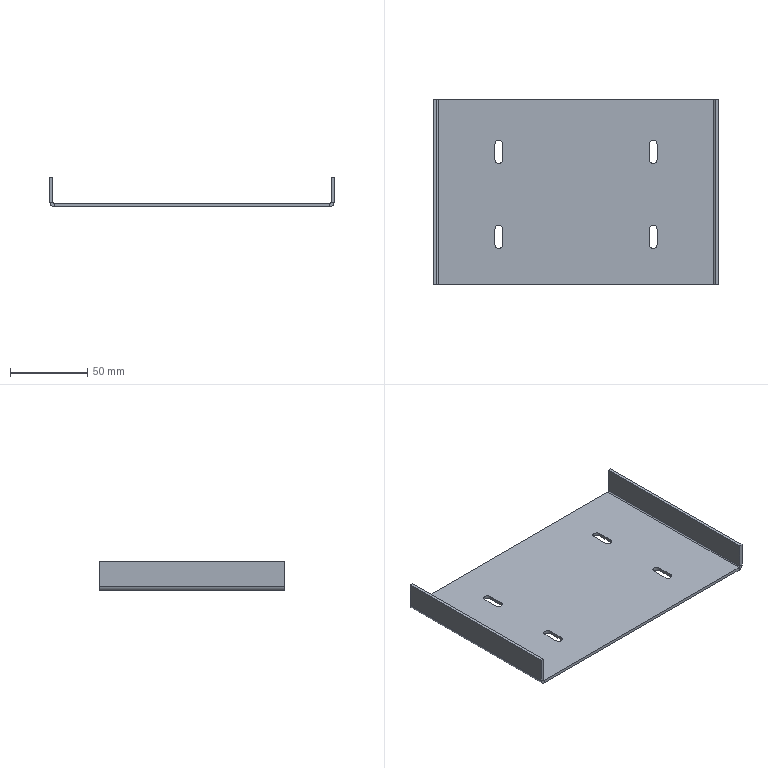Part | NX | 1 solid | 38 faces | box 184 x 120 x 19 mm | volume 51405 mm3 | plane 26 | cylinder 12 | commonest cylinder face diameters 5 x8 1.473 x2 5.473 x2
STEP:
#1=CARTESIAN_POINT('',(-89.263,185.5,-19.));
#2=VERTEX_POINT('',#1);
#3=CARTESIAN_POINT('',(-89.263,185.5,-21.));
#4=VERTEX_POINT('',#3);
#5=CARTESIAN_POINT('',(-89.263,185.5,-19.));
#6=DIRECTION('',(0.,0.,-1.));
#7=VECTOR('',#6,1000.);
#8=LINE('',#5,#7);
#9=EDGE_CURVE('',#2,#4,#8,.T.);
#10=ORIENTED_EDGE('',*,*,#9,.F.);
#11=CARTESIAN_POINT('',(-90.,185.5,-18.263));
#12=VERTEX_POINT('',#11);
#13=CARTESIAN_POINT('',(-89.263,185.5,-18.263));
#14=DIRECTION('',(0.,1.,0.));
#15=DIRECTION('',(-1.,0.,0.));
#16=AXIS2_PLACEMENT_3D('',#13,#14,#15);
#17=CIRCLE('',#16,0.7366);
#18=EDGE_CURVE('',#12,#2,#17,.F.);
#19=ORIENTED_EDGE('',*,*,#18,.F.);
#20=CARTESIAN_POINT('',(-92.,185.5,-18.263));
#21=VERTEX_POINT('',#20);
#22=CARTESIAN_POINT('',(-92.,185.5,-18.263));
#23=DIRECTION('',(1.,0.,0.));
#24=VECTOR('',#23,1000.);
#25=LINE('',#22,#24);
#26=EDGE_CURVE('',#21,#12,#25,.T.);
#27=ORIENTED_EDGE('',*,*,#26,.F.);
#28=CARTESIAN_POINT('',(-89.263,185.5,-18.263));
#29=DIRECTION('',(0.,-1.,0.));
#30=DIRECTION('',(1.,0.,0.));
#31=AXIS2_PLACEMENT_3D('',#28,#29,#30);
#32=CIRCLE('',#31,2.737);
#33=EDGE_CURVE('',#21,#4,#32,.T.);
#34=ORIENTED_EDGE('',*,*,#33,.T.);
#35=EDGE_LOOP('',(#10,#19,#27,#34));
#36=FACE_BOUND('',#35,.T.);
#37=CARTESIAN_POINT('',(-89.263,185.5,-19.));
#38=DIRECTION('',(0.,-1.,0.));
#39=DIRECTION('',(0.,0.,-1.));
#40=AXIS2_PLACEMENT_3D('',#37,#38,#39);
#41=PLANE('',#40);
#42=ADVANCED_FACE('',(#36),#41,.T.);
#43=CARTESIAN_POINT('',(89.263,185.5,-19.));
#44=VERTEX_POINT('',#43);
#45=CARTESIAN_POINT('',(-90.,185.5,-19.));
#46=DIRECTION('',(1.,0.,0.));
#47=VECTOR('',#46,1000.);
#48=LINE('',#45,#47);
#49=EDGE_CURVE('',#2,#44,#48,.T.);
#50=ORIENTED_EDGE('',*,*,#49,.F.);
#51=ORIENTED_EDGE('',*,*,#9,.T.);
#52=CARTESIAN_POINT('',(89.263,185.5,-21.));
#53=VERTEX_POINT('',#52);
#54=CARTESIAN_POINT('',(-90.,185.5,-21.));
#55=DIRECTION('',(1.,0.,0.));
#56=VECTOR('',#55,1000.);
#57=LINE('',#54,#56);
#58=EDGE_CURVE('',#4,#53,#57,.T.);
#59=ORIENTED_EDGE('',*,*,#58,.T.);
#60=CARTESIAN_POINT('',(89.263,185.5,-21.));
#61=DIRECTION('',(0.,0.,1.));
#62=VECTOR('',#61,1000.);
#63=LINE('',#60,#62);
#64=EDGE_CURVE('',#53,#44,#63,.T.);
#65=ORIENTED_EDGE('',*,*,#64,.T.);
#66=EDGE_LOOP('',(#50,#51,#59,#65));
#67=FACE_BOUND('',#66,.T.);
#68=CARTESIAN_POINT('',(-92.,185.5,-18.263));
#69=DIRECTION('',(0.,-1.,0.));
#70=DIRECTION('',(0.,0.,-1.));
#71=AXIS2_PLACEMENT_3D('',#68,#69,#70);
#72=PLANE('',#71);
#73=ADVANCED_FACE('',(#67),#72,.T.);
#74=CARTESIAN_POINT('',(-90.,305.5,-18.263));
#75=VERTEX_POINT('',#74);
#76=CARTESIAN_POINT('',(-92.,305.5,-18.263));
#77=VERTEX_POINT('',#76);
#78=CARTESIAN_POINT('',(-90.,305.5,-18.263));
#79=DIRECTION('',(-1.,0.,0.));
#80=VECTOR('',#79,1000.);
#81=LINE('',#78,#80);
#82=EDGE_CURVE('',#75,#77,#81,.T.);
#83=ORIENTED_EDGE('',*,*,#82,.F.);
#84=CARTESIAN_POINT('',(-89.263,305.5,-19.));
#85=VERTEX_POINT('',#84);
#86=CARTESIAN_POINT('',(-89.263,305.5,-18.263));
#87=DIRECTION('',(0.,1.,0.));
#88=DIRECTION('',(-1.,0.,0.));
#89=AXIS2_PLACEMENT_3D('',#86,#87,#88);
#90=CIRCLE('',#89,0.7366);
#91=EDGE_CURVE('',#75,#85,#90,.F.);
#92=ORIENTED_EDGE('',*,*,#91,.T.);
#93=CARTESIAN_POINT('',(-89.263,305.5,-21.));
#94=VERTEX_POINT('',#93);
#95=CARTESIAN_POINT('',(-89.263,305.5,-21.));
#96=DIRECTION('',(0.,0.,1.));
#97=VECTOR('',#96,1000.);
#98=LINE('',#95,#97);
#99=EDGE_CURVE('',#94,#85,#98,.T.);
#100=ORIENTED_EDGE('',*,*,#99,.F.);
#101=CARTESIAN_POINT('',(-89.263,305.5,-18.263));
#102=DIRECTION('',(0.,-1.,0.));
#103=DIRECTION('',(1.,0.,0.));
#104=AXIS2_PLACEMENT_3D('',#101,#102,#103);
#105=CIRCLE('',#104,2.737);
#106=EDGE_CURVE('',#77,#94,#105,.T.);
#107=ORIENTED_EDGE('',*,*,#106,.F.);
#108=EDGE_LOOP('',(#83,#92,#100,#107));
#109=FACE_BOUND('',#108,.T.);
#110=CARTESIAN_POINT('',(-90.,305.5,-18.263));
#111=DIRECTION('',(0.,1.,0.));
#112=DIRECTION('',(0.,0.,1.));
#113=AXIS2_PLACEMENT_3D('',#110,#111,#112);
#114=PLANE('',#113);
#115=ADVANCED_FACE('',(#109),#114,.T.);
#116=CARTESIAN_POINT('',(-90.,305.5,-2.));
#117=VERTEX_POINT('',#116);
#118=CARTESIAN_POINT('',(-90.,305.5,-2.));
#119=DIRECTION('',(0.,0.,-1.));
#120=VECTOR('',#119,1000.);
#121=LINE('',#118,#120);
#122=EDGE_CURVE('',#117,#75,#121,.T.);
#123=ORIENTED_EDGE('',*,*,#122,.T.);
#124=ORIENTED_EDGE('',*,*,#82,.T.);
#125=CARTESIAN_POINT('',(-92.,305.5,-2.));
#126=VERTEX_POINT('',#125);
#127=CARTESIAN_POINT('',(-92.,305.5,-2.));
#128=DIRECTION('',(0.,0.,1.));
#129=VECTOR('',#128,1000.);
#130=LINE('',#127,#129);
#131=EDGE_CURVE('',#126,#77,#130,.F.);
#132=ORIENTED_EDGE('',*,*,#131,.F.);
#133=CARTESIAN_POINT('',(-92.,305.5,-2.));
#134=DIRECTION('',(1.,0.,0.));
#135=VECTOR('',#134,1000.);
#136=LINE('',#133,#135);
#137=EDGE_CURVE('',#126,#117,#136,.T.);
#138=ORIENTED_EDGE('',*,*,#137,.T.);
#139=EDGE_LOOP('',(#123,#124,#132,#138));
#140=FACE_BOUND('',#139,.T.);
#141=CARTESIAN_POINT('',(-89.263,305.5,-21.));
#142=DIRECTION('',(0.,1.,0.));
#143=DIRECTION('',(0.,0.,1.));
#144=AXIS2_PLACEMENT_3D('',#141,#142,#143);
#145=PLANE('',#144);
#146=ADVANCED_FACE('',(#140),#145,.T.);
#147=CARTESIAN_POINT('',(90.,185.5,-18.263));
#148=VERTEX_POINT('',#147);
#149=CARTESIAN_POINT('',(92.,185.5,-18.263));
#150=VERTEX_POINT('',#149);
#151=CARTESIAN_POINT('',(90.,185.5,-18.263));
#152=DIRECTION('',(1.,0.,0.));
#153=VECTOR('',#152,1000.);
#154=LINE('',#151,#153);
#155=EDGE_CURVE('',#148,#150,#154,.T.);
#156=ORIENTED_EDGE('',*,*,#155,.F.);
#157=CARTESIAN_POINT('',(89.263,185.5,-18.263));
#158=DIRECTION('',(0.,1.,0.));
#159=DIRECTION('',(0.,0.,1.));
#160=AXIS2_PLACEMENT_3D('',#157,#158,#159);
#161=CIRCLE('',#160,0.7366);
#162=EDGE_CURVE('',#44,#148,#161,.F.);
#163=ORIENTED_EDGE('',*,*,#162,.F.);
#164=ORIENTED_EDGE('',*,*,#64,.F.);
#165=CARTESIAN_POINT('',(89.263,185.5,-18.263));
#166=DIRECTION('',(0.,-1.,0.));
#167=DIRECTION('',(1.,0.,0.));
#168=AXIS2_PLACEMENT_3D('',#165,#166,#167);
#169=CIRCLE('',#168,2.737);
#170=EDGE_CURVE('',#53,#150,#169,.T.);
#171=ORIENTED_EDGE('',*,*,#170,.T.);
#172=EDGE_LOOP('',(#156,#163,#164,#171));
#173=FACE_BOUND('',#172,.T.);
#174=CARTESIAN_POINT('',(90.,185.5,-18.263));
#175=DIRECTION('',(0.,-1.,0.));
#176=DIRECTION('',(0.,0.,-1.));
#177=AXIS2_PLACEMENT_3D('',#174,#175,#176);
#178=PLANE('',#177);
#179=ADVANCED_FACE('',(#173),#178,.T.);
#180=CARTESIAN_POINT('',(90.,185.5,-2.));
#181=VERTEX_POINT('',#180);
#182=CARTESIAN_POINT('',(90.,185.5,-19.));
#183=DIRECTION('',(0.,0.,1.));
#184=VECTOR('',#183,1000.);
#185=LINE('',#182,#184);
#186=EDGE_CURVE('',#148,#181,#185,.T.);
#187=ORIENTED_EDGE('',*,*,#186,.F.);
#188=ORIENTED_EDGE('',*,*,#155,.T.);
#189=CARTESIAN_POINT('',(92.,185.5,-2.));
#190=VERTEX_POINT('',#189);
#191=CARTESIAN_POINT('',(92.,185.5,-19.));
#192=DIRECTION('',(0.,0.,1.));
#193=VECTOR('',#192,1000.);
#194=LINE('',#191,#193);
#195=EDGE_CURVE('',#150,#190,#194,.T.);
#196=ORIENTED_EDGE('',*,*,#195,.T.);
#197=CARTESIAN_POINT('',(90.,185.5,-2.));
#198=DIRECTION('',(1.,0.,0.));
#199=VECTOR('',#198,1000.);
#200=LINE('',#197,#199);
#201=EDGE_CURVE('',#181,#190,#200,.T.);
#202=ORIENTED_EDGE('',*,*,#201,.F.);
#203=EDGE_LOOP('',(#187,#188,#196,#202));
#204=FACE_BOUND('',#203,.T.);
#205=CARTESIAN_POINT('',(89.263,185.5,-21.));
#206=DIRECTION('',(0.,-1.,0.));
#207=DIRECTION('',(0.,0.,-1.));
#208=AXIS2_PLACEMENT_3D('',#205,#206,#207);
#209=PLANE('',#208);
#210=ADVANCED_FACE('',(#204),#209,.T.);
#211=CARTESIAN_POINT('',(89.263,305.5,-19.));
#212=VERTEX_POINT('',#211);
#213=CARTESIAN_POINT('',(89.263,305.5,-21.));
#214=VERTEX_POINT('',#213);
#215=CARTESIAN_POINT('',(89.263,305.5,-19.));
#216=DIRECTION('',(0.,0.,-1.));
#217=VECTOR('',#216,1000.);
#218=LINE('',#215,#217);
#219=EDGE_CURVE('',#212,#214,#218,.T.);
#220=ORIENTED_EDGE('',*,*,#219,.F.);
#221=CARTESIAN_POINT('',(90.,305.5,-18.263));
#222=VERTEX_POINT('',#221);
#223=CARTESIAN_POINT('',(89.263,305.5,-18.263));
#224=DIRECTION('',(0.,1.,0.));
#225=DIRECTION('',(0.,0.,1.));
#226=AXIS2_PLACEMENT_3D('',#223,#224,#225);
#227=CIRCLE('',#226,0.7366);
#228=EDGE_CURVE('',#212,#222,#227,.F.);
#229=ORIENTED_EDGE('',*,*,#228,.T.);
#230=CARTESIAN_POINT('',(92.,305.5,-18.263));
#231=VERTEX_POINT('',#230);
#232=CARTESIAN_POINT('',(92.,305.5,-18.263));
#233=DIRECTION('',(-1.,0.,0.));
#234=VECTOR('',#233,1000.);
#235=LINE('',#232,#234);
#236=EDGE_CURVE('',#231,#222,#235,.T.);
#237=ORIENTED_EDGE('',*,*,#236,.F.);
#238=CARTESIAN_POINT('',(89.263,305.5,-18.263));
#239=DIRECTION('',(0.,-1.,0.));
#240=DIRECTION('',(1.,0.,0.));
#241=AXIS2_PLACEMENT_3D('',#238,#239,#240);
#242=CIRCLE('',#241,2.737);
#243=EDGE_CURVE('',#214,#231,#242,.T.);
#244=ORIENTED_EDGE('',*,*,#243,.F.);
#245=EDGE_LOOP('',(#220,#229,#237,#244));
#246=FACE_BOUND('',#245,.T.);
#247=CARTESIAN_POINT('',(89.263,305.5,-19.));
#248=DIRECTION('',(0.,1.,0.));
#249=DIRECTION('',(0.,0.,1.));
#250=AXIS2_PLACEMENT_3D('',#247,#248,#249);
#251=PLANE('',#250);
#252=ADVANCED_FACE('',(#246),#251,.T.);
#253=CARTESIAN_POINT('',(-90.,305.5,-19.));
#254=DIRECTION('',(1.,0.,0.));
#255=VECTOR('',#254,1000.);
#256=LINE('',#253,#255);
#257=EDGE_CURVE('',#85,#212,#256,.T.);
#258=ORIENTED_EDGE('',*,*,#257,.T.);
#259=ORIENTED_EDGE('',*,*,#219,.T.);
#260=CARTESIAN_POINT('',(-90.,305.5,-21.));
#261=DIRECTION('',(1.,0.,0.));
#262=VECTOR('',#261,1000.);
#263=LINE('',#260,#262);
#264=EDGE_CURVE('',#94,#214,#263,.T.);
#265=ORIENTED_EDGE('',*,*,#264,.F.);
#266=ORIENTED_EDGE('',*,*,#99,.T.);
#267=EDGE_LOOP('',(#258,#259,#265,#266));
#268=FACE_BOUND('',#267,.T.);
#269=CARTESIAN_POINT('',(92.,305.5,-18.263));
#270=DIRECTION('',(0.,1.,0.));
#271=DIRECTION('',(0.,0.,1.));
#272=AXIS2_PLACEMENT_3D('',#269,#270,#271);
#273=PLANE('',#272);
#274=ADVANCED_FACE('',(#268),#273,.T.);
#275=CARTESIAN_POINT('',(92.,305.5,-2.));
#276=VERTEX_POINT('',#275);
#277=CARTESIAN_POINT('',(92.,305.5,-19.));
#278=DIRECTION('',(0.,0.,1.));
#279=VECTOR('',#278,1000.);
#280=LINE('',#277,#279);
#281=EDGE_CURVE('',#231,#276,#280,.T.);
#282=ORIENTED_EDGE('',*,*,#281,.T.);
#283=CARTESIAN_POINT('',(92.,185.5,-2.));
#284=DIRECTION('',(0.,1.,0.));
#285=VECTOR('',#284,1000.);
#286=LINE('',#283,#285);
#287=EDGE_CURVE('',#190,#276,#286,.T.);
#288=ORIENTED_EDGE('',*,*,#287,.F.);
#289=ORIENTED_EDGE('',*,*,#195,.F.);
#290=CARTESIAN_POINT('',(92.,185.5,-18.263));
#291=DIRECTION('',(0.,1.,0.));
#292=VECTOR('',#291,1000.);
#293=LINE('',#290,#292);
#294=EDGE_CURVE('',#150,#231,#293,.T.);
#295=ORIENTED_EDGE('',*,*,#294,.T.);
#296=EDGE_LOOP('',(#282,#288,#289,#295));
#297=FACE_BOUND('',#296,.T.);
#298=CARTESIAN_POINT('',(92.,185.5,-19.));
#299=DIRECTION('',(-1.,0.,0.));
#300=DIRECTION('',(0.,0.,1.));
#301=AXIS2_PLACEMENT_3D('',#298,#299,#300);
#302=PLANE('',#301);
#303=ADVANCED_FACE('',(#297),#302,.F.);
#304=CARTESIAN_POINT('',(90.,305.5,-2.));
#305=VERTEX_POINT('',#304);
#306=CARTESIAN_POINT('',(90.,305.5,-2.));
#307=DIRECTION('',(1.,0.,0.));
#308=VECTOR('',#307,1000.);
#309=LINE('',#306,#308);
#310=EDGE_CURVE('',#305,#276,#309,.T.);
#311=ORIENTED_EDGE('',*,*,#310,.F.);
#312=CARTESIAN_POINT('',(90.,185.5,-2.));
#313=DIRECTION('',(0.,1.,0.));
#314=VECTOR('',#313,1000.);
#315=LINE('',#312,#314);
#316=EDGE_CURVE('',#181,#305,#315,.T.);
#317=ORIENTED_EDGE('',*,*,#316,.F.);
#318=ORIENTED_EDGE('',*,*,#201,.T.);
#319=ORIENTED_EDGE('',*,*,#287,.T.);
#320=EDGE_LOOP('',(#311,#317,#318,#319));
#321=FACE_BOUND('',#320,.T.);
#322=CARTESIAN_POINT('',(90.,185.5,-2.));
#323=DIRECTION('',(0.,0.,1.));
#324=DIRECTION('',(1.,0.,0.));
#325=AXIS2_PLACEMENT_3D('',#322,#323,#324);
#326=PLANE('',#325);
#327=ADVANCED_FACE('',(#321),#326,.T.);
#328=CARTESIAN_POINT('',(90.,305.5,-19.));
#329=DIRECTION('',(0.,0.,1.));
#330=VECTOR('',#329,1000.);
#331=LINE('',#328,#330);
#332=EDGE_CURVE('',#222,#305,#331,.T.);
#333=ORIENTED_EDGE('',*,*,#332,.F.);
#334=CARTESIAN_POINT('',(90.,185.5,-18.263));
#335=DIRECTION('',(0.,1.,0.));
#336=VECTOR('',#335,1000.);
#337=LINE('',#334,#336);
#338=EDGE_CURVE('',#148,#222,#337,.T.);
#339=ORIENTED_EDGE('',*,*,#338,.F.);
#340=ORIENTED_EDGE('',*,*,#186,.T.);
#341=ORIENTED_EDGE('',*,*,#316,.T.);
#342=EDGE_LOOP('',(#333,#339,#340,#341));
#343=FACE_BOUND('',#342,.T.);
#344=CARTESIAN_POINT('',(90.,185.5,-19.));
#345=DIRECTION('',(-1.,0.,0.));
#346=DIRECTION('',(0.,0.,1.));
#347=AXIS2_PLACEMENT_3D('',#344,#345,#346);
#348=PLANE('',#347);
#349=ADVANCED_FACE('',(#343),#348,.T.);
#350=ORIENTED_EDGE('',*,*,#228,.F.);
#351=CARTESIAN_POINT('',(89.263,185.5,-19.));
#352=DIRECTION('',(0.,1.,0.));
#353=VECTOR('',#352,1000.);
#354=LINE('',#351,#353);
#355=EDGE_CURVE('',#44,#212,#354,.T.);
#356=ORIENTED_EDGE('',*,*,#355,.F.);
#357=ORIENTED_EDGE('',*,*,#162,.T.);
#358=ORIENTED_EDGE('',*,*,#338,.T.);
#359=EDGE_LOOP('',(#350,#356,#357,#358));
#360=FACE_BOUND('',#359,.T.);
#361=CARTESIAN_POINT('',(89.263,185.5,-18.263));
#362=DIRECTION('',(0.,1.,0.));
#363=DIRECTION('',(-1.,0.,0.));
#364=AXIS2_PLACEMENT_3D('',#361,#362,#363);
#365=CYLINDRICAL_SURFACE('',#364,0.7366);
#366=ADVANCED_FACE('',(#360),#365,.F.);
#367=CARTESIAN_POINT('',(-52.5,221.5,-19.));
#368=VERTEX_POINT('',#367);
#369=CARTESIAN_POINT('',(-47.5,221.5,-19.));
#370=VERTEX_POINT('',#369);
#371=CARTESIAN_POINT('',(-50.,221.5,-19.));
#372=DIRECTION('',(0.,0.,-1.));
#373=DIRECTION('',(-1.,0.,0.));
#374=AXIS2_PLACEMENT_3D('',#371,#372,#373);
#375=CIRCLE('',#374,2.5);
#376=EDGE_CURVE('',#368,#370,#375,.T.);
#377=ORIENTED_EDGE('',*,*,#376,.T.);
#378=CARTESIAN_POINT('',(-47.5,211.5,-19.));
#379=VERTEX_POINT('',#378);
#380=CARTESIAN_POINT('',(-47.5,221.5,-19.));
#381=DIRECTION('',(0.,-1.,0.));
#382=VECTOR('',#381,1000.);
#383=LINE('',#380,#382);
#384=EDGE_CURVE('',#370,#379,#383,.T.);
#385=ORIENTED_EDGE('',*,*,#384,.T.);
#386=CARTESIAN_POINT('',(-52.5,211.5,-19.));
#387=VERTEX_POINT('',#386);
#388=CARTESIAN_POINT('',(-50.,211.5,-19.));
#389=DIRECTION('',(0.,0.,-1.));
#390=DIRECTION('',(-1.,0.,0.));
#391=AXIS2_PLACEMENT_3D('',#388,#389,#390);
#392=CIRCLE('',#391,2.5);
#393=EDGE_CURVE('',#379,#387,#392,.T.);
#394=ORIENTED_EDGE('',*,*,#393,.T.);
#395=CARTESIAN_POINT('',(-52.5,221.5,-19.));
#396=DIRECTION('',(0.,1.,0.));
#397=VECTOR('',#396,1000.);
#398=LINE('',#395,#397);
#399=EDGE_CURVE('',#387,#368,#398,.T.);
#400=ORIENTED_EDGE('',*,*,#399,.T.);
#401=EDGE_LOOP('',(#377,#385,#394,#400));
#402=FACE_BOUND('',#401,.T.);
#403=CARTESIAN_POINT('',(47.5,221.5,-19.));
#404=VERTEX_POINT('',#403);
#405=CARTESIAN_POINT('',(52.5,221.5,-19.));
#406=VERTEX_POINT('',#405);
#407=CARTESIAN_POINT('',(50.,221.5,-19.));
#408=DIRECTION('',(0.,0.,-1.));
#409=DIRECTION('',(-1.,0.,0.));
#410=AXIS2_PLACEMENT_3D('',#407,#408,#409);
#411=CIRCLE('',#410,2.5);
#412=EDGE_CURVE('',#404,#406,#411,.T.);
#413=ORIENTED_EDGE('',*,*,#412,.T.);
#414=CARTESIAN_POINT('',(52.5,211.5,-19.));
#415=VERTEX_POINT('',#414);
#416=CARTESIAN_POINT('',(52.5,221.5,-19.));
#417=DIRECTION('',(0.,-1.,0.));
#418=VECTOR('',#417,1000.);
#419=LINE('',#416,#418);
#420=EDGE_CURVE('',#406,#415,#419,.T.);
#421=ORIENTED_EDGE('',*,*,#420,.T.);
#422=CARTESIAN_POINT('',(47.5,211.5,-19.));
#423=VERTEX_POINT('',#422);
#424=CARTESIAN_POINT('',(50.,211.5,-19.));
#425=DIRECTION('',(0.,0.,-1.));
#426=DIRECTION('',(-1.,0.,0.));
#427=AXIS2_PLACEMENT_3D('',#424,#425,#426);
#428=CIRCLE('',#427,2.5);
#429=EDGE_CURVE('',#415,#423,#428,.T.);
#430=ORIENTED_EDGE('',*,*,#429,.T.);
#431=CARTESIAN_POINT('',(47.5,221.5,-19.));
#432=DIRECTION('',(0.,1.,0.));
#433=VECTOR('',#432,1000.);
#434=LINE('',#431,#433);
#435=EDGE_CURVE('',#423,#404,#434,.T.);
#436=ORIENTED_EDGE('',*,*,#435,.T.);
#437=EDGE_LOOP('',(#413,#421,#430,#436));
#438=FACE_BOUND('',#437,.T.);
#439=CARTESIAN_POINT('',(-52.5,276.5,-19.));
#440=VERTEX_POINT('',#439);
#441=CARTESIAN_POINT('',(-47.5,276.5,-19.));
#442=VERTEX_POINT('',#441);
#443=CARTESIAN_POINT('',(-50.,276.5,-19.));
#444=DIRECTION('',(0.,0.,-1.));
#445=DIRECTION('',(-1.,0.,0.));
#446=AXIS2_PLACEMENT_3D('',#443,#444,#445);
#447=CIRCLE('',#446,2.5);
#448=EDGE_CURVE('',#440,#442,#447,.T.);
#449=ORIENTED_EDGE('',*,*,#448,.T.);
#450=CARTESIAN_POINT('',(-47.5,266.5,-19.));
#451=VERTEX_POINT('',#450);
#452=CARTESIAN_POINT('',(-47.5,276.5,-19.));
#453=DIRECTION('',(0.,-1.,0.));
#454=VECTOR('',#453,1000.);
#455=LINE('',#452,#454);
#456=EDGE_CURVE('',#442,#451,#455,.T.);
#457=ORIENTED_EDGE('',*,*,#456,.T.);
#458=CARTESIAN_POINT('',(-52.5,266.5,-19.));
#459=VERTEX_POINT('',#458);
#460=CARTESIAN_POINT('',(-50.,266.5,-19.));
#461=DIRECTION('',(0.,0.,-1.));
#462=DIRECTION('',(-1.,0.,0.));
#463=AXIS2_PLACEMENT_3D('',#460,#461,#462);
#464=CIRCLE('',#463,2.5);
#465=EDGE_CURVE('',#451,#459,#464,.T.);
#466=ORIENTED_EDGE('',*,*,#465,.T.);
#467=CARTESIAN_POINT('',(-52.5,276.5,-19.));
#468=DIRECTION('',(0.,1.,0.));
#469=VECTOR('',#468,1000.);
#470=LINE('',#467,#469);
#471=EDGE_CURVE('',#459,#440,#470,.T.);
#472=ORIENTED_EDGE('',*,*,#471,.T.);
#473=EDGE_LOOP('',(#449,#457,#466,#472));
#474=FACE_BOUND('',#473,.T.);
#475=CARTESIAN_POINT('',(47.5,276.5,-19.));
#476=VERTEX_POINT('',#475);
#477=CARTESIAN_POINT('',(52.5,276.5,-19.));
#478=VERTEX_POINT('',#477);
#479=CARTESIAN_POINT('',(50.,276.5,-19.));
#480=DIRECTION('',(0.,0.,-1.));
#481=DIRECTION('',(-1.,0.,0.));
#482=AXIS2_PLACEMENT_3D('',#479,#480,#481);
#483=CIRCLE('',#482,2.5);
#484=EDGE_CURVE('',#476,#478,#483,.T.);
#485=ORIENTED_EDGE('',*,*,#484,.T.);
#486=CARTESIAN_POINT('',(52.5,266.5,-19.));
#487=VERTEX_POINT('',#486);
#488=CARTESIAN_POINT('',(52.5,276.5,-19.));
#489=DIRECTION('',(0.,-1.,0.));
#490=VECTOR('',#489,1000.);
#491=LINE('',#488,#490);
#492=EDGE_CURVE('',#478,#487,#491,.T.);
#493=ORIENTED_EDGE('',*,*,#492,.T.);
#494=CARTESIAN_POINT('',(47.5,266.5,-19.));
#495=VERTEX_POINT('',#494);
#496=CARTESIAN_POINT('',(50.,266.5,-19.));
#497=DIRECTION('',(0.,0.,-1.));
#498=DIRECTION('',(-1.,0.,0.));
#499=AXIS2_PLACEMENT_3D('',#496,#497,#498);
#500=CIRCLE('',#499,2.5);
#501=EDGE_CURVE('',#487,#495,#500,.T.);
#502=ORIENTED_EDGE('',*,*,#501,.T.);
#503=CARTESIAN_POINT('',(47.5,276.5,-19.));
#504=DIRECTION('',(0.,1.,0.));
#505=VECTOR('',#504,1000.);
#506=LINE('',#503,#505);
#507=EDGE_CURVE('',#495,#476,#506,.T.);
#508=ORIENTED_EDGE('',*,*,#507,.T.);
#509=EDGE_LOOP('',(#485,#493,#502,#508));
#510=FACE_BOUND('',#509,.T.);
#511=ORIENTED_EDGE('',*,*,#257,.F.);
#512=CARTESIAN_POINT('',(-89.263,185.5,-19.));
#513=DIRECTION('',(0.,1.,0.));
#514=VECTOR('',#513,1000.);
#515=LINE('',#512,#514);
#516=EDGE_CURVE('',#2,#85,#515,.T.);
#517=ORIENTED_EDGE('',*,*,#516,.F.);
#518=ORIENTED_EDGE('',*,*,#49,.T.);
#519=ORIENTED_EDGE('',*,*,#355,.T.);
#520=EDGE_LOOP('',(#511,#517,#518,#519));
#521=FACE_BOUND('',#520,.T.);
#522=CARTESIAN_POINT('',(-90.,185.5,-19.));
#523=DIRECTION('',(0.,0.,1.));
#524=DIRECTION('',(1.,0.,0.));
#525=AXIS2_PLACEMENT_3D('',#522,#523,#524);
#526=PLANE('',#525);
#527=ADVANCED_FACE('',(#402,#438,#474,#510,#521),#526,.T.);
#528=ORIENTED_EDGE('',*,*,#91,.F.);
#529=CARTESIAN_POINT('',(-90.,185.5,-18.263));
#530=DIRECTION('',(0.,1.,0.));
#531=VECTOR('',#530,1000.);
#532=LINE('',#529,#531);
#533=EDGE_CURVE('',#12,#75,#532,.T.);
#534=ORIENTED_EDGE('',*,*,#533,.F.);
#535=ORIENTED_EDGE('',*,*,#18,.T.);
#536=ORIENTED_EDGE('',*,*,#516,.T.);
#537=EDGE_LOOP('',(#528,#534,#535,#536));
#538=FACE_BOUND('',#537,.T.);
#539=CARTESIAN_POINT('',(-89.263,185.5,-18.263));
#540=DIRECTION('',(0.,1.,0.));
#541=DIRECTION('',(-1.,0.,0.));
#542=AXIS2_PLACEMENT_3D('',#539,#540,#541);
#543=CYLINDRICAL_SURFACE('',#542,0.7366);
#544=ADVANCED_FACE('',(#538),#543,.F.);
#545=ORIENTED_EDGE('',*,*,#122,.F.);
#546=CARTESIAN_POINT('',(-90.,185.5,-2.));
#547=VERTEX_POINT('',#546);
#548=CARTESIAN_POINT('',(-90.,185.5,-2.));
#549=DIRECTION('',(0.,1.,0.));
#550=VECTOR('',#549,1000.);
#551=LINE('',#548,#550);
#552=EDGE_CURVE('',#547,#117,#551,.T.);
#553=ORIENTED_EDGE('',*,*,#552,.F.);
#554=CARTESIAN_POINT('',(-90.,185.5,-2.));
#555=DIRECTION('',(0.,0.,-1.));
#556=VECTOR('',#555,1000.);
#557=LINE('',#554,#556);
#558=EDGE_CURVE('',#547,#12,#557,.T.);
#559=ORIENTED_EDGE('',*,*,#558,.T.);
#560=ORIENTED_EDGE('',*,*,#533,.T.);
#561=EDGE_LOOP('',(#545,#553,#559,#560));
#562=FACE_BOUND('',#561,.T.);
#563=CARTESIAN_POINT('',(-90.,185.5,-2.));
#564=DIRECTION('',(1.,0.,0.));
#565=DIRECTION('',(0.,1.,0.));
#566=AXIS2_PLACEMENT_3D('',#563,#564,#565);
#567=PLANE('',#566);
#568=ADVANCED_FACE('',(#562),#567,.T.);
#569=ORIENTED_EDGE('',*,*,#137,.F.);
#570=CARTESIAN_POINT('',(-92.,185.5,-2.));
#571=VERTEX_POINT('',#570);
#572=CARTESIAN_POINT('',(-92.,185.5,-2.));
#573=DIRECTION('',(0.,1.,0.));
#574=VECTOR('',#573,1000.);
#575=LINE('',#572,#574);
#576=EDGE_CURVE('',#571,#126,#575,.T.);
#577=ORIENTED_EDGE('',*,*,#576,.F.);
#578=CARTESIAN_POINT('',(-92.,185.5,-2.));
#579=DIRECTION('',(1.,0.,0.));
#580=VECTOR('',#579,1000.);
#581=LINE('',#578,#580);
#582=EDGE_CURVE('',#571,#547,#581,.T.);
#583=ORIENTED_EDGE('',*,*,#582,.T.);
#584=ORIENTED_EDGE('',*,*,#552,.T.);
#585=EDGE_LOOP('',(#569,#577,#583,#584));
#586=FACE_BOUND('',#585,.T.);
#587=CARTESIAN_POINT('',(-92.,185.5,-2.));
#588=DIRECTION('',(0.,0.,1.));
#589=DIRECTION('',(1.,0.,0.));
#590=AXIS2_PLACEMENT_3D('',#587,#588,#589);
#591=PLANE('',#590);
#592=ADVANCED_FACE('',(#586),#591,.T.);
#593=ORIENTED_EDGE('',*,*,#131,.T.);
#594=CARTESIAN_POINT('',(-92.,185.5,-18.263));
#595=DIRECTION('',(0.,1.,0.));
#596=VECTOR('',#595,1000.);
#597=LINE('',#594,#596);
#598=EDGE_CURVE('',#21,#77,#597,.T.);
#599=ORIENTED_EDGE('',*,*,#598,.F.);
#600=CARTESIAN_POINT('',(-92.,185.5,-2.));
#601=DIRECTION('',(0.,0.,1.));
#602=VECTOR('',#601,1000.);
#603=LINE('',#600,#602);
#604=EDGE_CURVE('',#571,#21,#603,.F.);
#605=ORIENTED_EDGE('',*,*,#604,.F.);
#606=ORIENTED_EDGE('',*,*,#576,.T.);
#607=EDGE_LOOP('',(#593,#599,#605,#606));
#608=FACE_BOUND('',#607,.T.);
#609=CARTESIAN_POINT('',(-92.,185.5,-2.));
#610=DIRECTION('',(1.,0.,0.));
#611=DIRECTION('',(0.,1.,0.));
#612=AXIS2_PLACEMENT_3D('',#609,#610,#611);
#613=PLANE('',#612);
#614=ADVANCED_FACE('',(#608),#613,.F.);
#615=ORIENTED_EDGE('',*,*,#106,.T.);
#616=CARTESIAN_POINT('',(-89.263,185.5,-21.));
#617=DIRECTION('',(0.,1.,0.));
#618=VECTOR('',#617,1000.);
#619=LINE('',#616,#618);
#620=EDGE_CURVE('',#4,#94,#619,.T.);
#621=ORIENTED_EDGE('',*,*,#620,.F.);
#622=ORIENTED_EDGE('',*,*,#33,.F.);
#623=ORIENTED_EDGE('',*,*,#598,.T.);
#624=EDGE_LOOP('',(#615,#621,#622,#623));
#625=FACE_BOUND('',#624,.T.);
#626=CARTESIAN_POINT('',(-89.263,185.5,-18.263));
#627=DIRECTION('',(0.,1.,0.));
#628=DIRECTION('',(-1.,0.,0.));
#629=AXIS2_PLACEMENT_3D('',#626,#627,#628);
#630=CYLINDRICAL_SURFACE('',#629,2.737);
#631=ADVANCED_FACE('',(#625),#630,.T.);
#632=CARTESIAN_POINT('',(-47.5,221.5,-21.));
#633=VERTEX_POINT('',#632);
#634=CARTESIAN_POINT('',(-47.5,211.5,-21.));
#635=VERTEX_POINT('',#634);
#636=CARTESIAN_POINT('',(-47.5,221.5,-21.));
#637=DIRECTION('',(0.,-1.,0.));
#638=VECTOR('',#637,1000.);
#639=LINE('',#636,#638);
#640=EDGE_CURVE('',#633,#635,#639,.T.);
#641=ORIENTED_EDGE('',*,*,#640,.F.);
#642=CARTESIAN_POINT('',(-52.5,221.5,-21.));
#643=VERTEX_POINT('',#642);
#644=CARTESIAN_POINT('',(-50.,221.5,-21.));
#645=DIRECTION('',(0.,0.,-1.));
#646=DIRECTION('',(-1.,0.,0.));
#647=AXIS2_PLACEMENT_3D('',#644,#645,#646);
#648=CIRCLE('',#647,2.5);
#649=EDGE_CURVE('',#643,#633,#648,.T.);
#650=ORIENTED_EDGE('',*,*,#649,.F.);
#651=CARTESIAN_POINT('',(-52.5,211.5,-21.));
#652=VERTEX_POINT('',#651);
#653=CARTESIAN_POINT('',(-52.5,221.5,-21.));
#654=DIRECTION('',(0.,1.,0.));
#655=VECTOR('',#654,1000.);
#656=LINE('',#653,#655);
#657=EDGE_CURVE('',#652,#643,#656,.T.);
#658=ORIENTED_EDGE('',*,*,#657,.F.);
#659=CARTESIAN_POINT('',(-50.,211.5,-21.));
#660=DIRECTION('',(0.,0.,-1.));
#661=DIRECTION('',(-1.,0.,0.));
#662=AXIS2_PLACEMENT_3D('',#659,#660,#661);
#663=CIRCLE('',#662,2.5);
#664=EDGE_CURVE('',#635,#652,#663,.T.);
#665=ORIENTED_EDGE('',*,*,#664,.F.);
#666=EDGE_LOOP('',(#641,#650,#658,#665));
#667=FACE_BOUND('',#666,.T.);
#668=CARTESIAN_POINT('',(52.5,221.5,-21.));
#669=VERTEX_POINT('',#668);
#670=CARTESIAN_POINT('',(52.5,211.5,-21.));
#671=VERTEX_POINT('',#670);
#672=CARTESIAN_POINT('',(52.5,221.5,-21.));
#673=DIRECTION('',(0.,-1.,0.));
#674=VECTOR('',#673,1000.);
#675=LINE('',#672,#674);
#676=EDGE_CURVE('',#669,#671,#675,.T.);
#677=ORIENTED_EDGE('',*,*,#676,.F.);
#678=CARTESIAN_POINT('',(47.5,221.5,-21.));
#679=VERTEX_POINT('',#678);
#680=CARTESIAN_POINT('',(50.,221.5,-21.));
#681=DIRECTION('',(0.,0.,-1.));
#682=DIRECTION('',(-1.,0.,0.));
#683=AXIS2_PLACEMENT_3D('',#680,#681,#682);
#684=CIRCLE('',#683,2.5);
#685=EDGE_CURVE('',#679,#669,#684,.T.);
#686=ORIENTED_EDGE('',*,*,#685,.F.);
#687=CARTESIAN_POINT('',(47.5,211.5,-21.));
#688=VERTEX_POINT('',#687);
#689=CARTESIAN_POINT('',(47.5,221.5,-21.));
#690=DIRECTION('',(0.,1.,0.));
#691=VECTOR('',#690,1000.);
#692=LINE('',#689,#691);
#693=EDGE_CURVE('',#688,#679,#692,.T.);
#694=ORIENTED_EDGE('',*,*,#693,.F.);
#695=CARTESIAN_POINT('',(50.,211.5,-21.));
#696=DIRECTION('',(0.,0.,-1.));
#697=DIRECTION('',(-1.,0.,0.));
#698=AXIS2_PLACEMENT_3D('',#695,#696,#697);
#699=CIRCLE('',#698,2.5);
#700=EDGE_CURVE('',#671,#688,#699,.T.);
#701=ORIENTED_EDGE('',*,*,#700,.F.);
#702=EDGE_LOOP('',(#677,#686,#694,#701));
#703=FACE_BOUND('',#702,.T.);
#704=CARTESIAN_POINT('',(-47.5,276.5,-21.));
#705=VERTEX_POINT('',#704);
#706=CARTESIAN_POINT('',(-47.5,266.5,-21.));
#707=VERTEX_POINT('',#706);
#708=CARTESIAN_POINT('',(-47.5,276.5,-21.));
#709=DIRECTION('',(0.,-1.,0.));
#710=VECTOR('',#709,1000.);
#711=LINE('',#708,#710);
#712=EDGE_CURVE('',#705,#707,#711,.T.);
#713=ORIENTED_EDGE('',*,*,#712,.F.);
#714=CARTESIAN_POINT('',(-52.5,276.5,-21.));
#715=VERTEX_POINT('',#714);
#716=CARTESIAN_POINT('',(-50.,276.5,-21.));
#717=DIRECTION('',(0.,0.,-1.));
#718=DIRECTION('',(-1.,0.,0.));
#719=AXIS2_PLACEMENT_3D('',#716,#717,#718);
#720=CIRCLE('',#719,2.5);
#721=EDGE_CURVE('',#715,#705,#720,.T.);
#722=ORIENTED_EDGE('',*,*,#721,.F.);
#723=CARTESIAN_POINT('',(-52.5,266.5,-21.));
#724=VERTEX_POINT('',#723);
#725=CARTESIAN_POINT('',(-52.5,276.5,-21.));
#726=DIRECTION('',(0.,1.,0.));
#727=VECTOR('',#726,1000.);
#728=LINE('',#725,#727);
#729=EDGE_CURVE('',#724,#715,#728,.T.);
#730=ORIENTED_EDGE('',*,*,#729,.F.);
#731=CARTESIAN_POINT('',(-50.,266.5,-21.));
#732=DIRECTION('',(0.,0.,-1.));
#733=DIRECTION('',(-1.,0.,0.));
#734=AXIS2_PLACEMENT_3D('',#731,#732,#733);
#735=CIRCLE('',#734,2.5);
#736=EDGE_CURVE('',#707,#724,#735,.T.);
#737=ORIENTED_EDGE('',*,*,#736,.F.);
#738=EDGE_LOOP('',(#713,#722,#730,#737));
#739=FACE_BOUND('',#738,.T.);
#740=CARTESIAN_POINT('',(52.5,276.5,-21.));
#741=VERTEX_POINT('',#740);
#742=CARTESIAN_POINT('',(52.5,266.5,-21.));
#743=VERTEX_POINT('',#742);
#744=CARTESIAN_POINT('',(52.5,276.5,-21.));
#745=DIRECTION('',(0.,-1.,0.));
#746=VECTOR('',#745,1000.);
#747=LINE('',#744,#746);
#748=EDGE_CURVE('',#741,#743,#747,.T.);
#749=ORIENTED_EDGE('',*,*,#748,.F.);
#750=CARTESIAN_POINT('',(47.5,276.5,-21.));
#751=VERTEX_POINT('',#750);
#752=CARTESIAN_POINT('',(50.,276.5,-21.));
#753=DIRECTION('',(0.,0.,-1.));
#754=DIRECTION('',(-1.,0.,0.));
#755=AXIS2_PLACEMENT_3D('',#752,#753,#754);
#756=CIRCLE('',#755,2.5);
#757=EDGE_CURVE('',#751,#741,#756,.T.);
#758=ORIENTED_EDGE('',*,*,#757,.F.);
#759=CARTESIAN_POINT('',(47.5,266.5,-21.));
#760=VERTEX_POINT('',#759);
#761=CARTESIAN_POINT('',(47.5,276.5,-21.));
#762=DIRECTION('',(0.,1.,0.));
#763=VECTOR('',#762,1000.);
#764=LINE('',#761,#763);
#765=EDGE_CURVE('',#760,#751,#764,.T.);
#766=ORIENTED_EDGE('',*,*,#765,.F.);
#767=CARTESIAN_POINT('',(50.,266.5,-21.));
#768=DIRECTION('',(0.,0.,-1.));
#769=DIRECTION('',(-1.,0.,0.));
#770=AXIS2_PLACEMENT_3D('',#767,#768,#769);
#771=CIRCLE('',#770,2.5);
#772=EDGE_CURVE('',#743,#760,#771,.T.);
#773=ORIENTED_EDGE('',*,*,#772,.F.);
#774=EDGE_LOOP('',(#749,#758,#766,#773));
#775=FACE_BOUND('',#774,.T.);
#776=ORIENTED_EDGE('',*,*,#264,.T.);
#777=CARTESIAN_POINT('',(89.263,185.5,-21.));
#778=DIRECTION('',(0.,1.,0.));
#779=VECTOR('',#778,1000.);
#780=LINE('',#777,#779);
#781=EDGE_CURVE('',#53,#214,#780,.T.);
#782=ORIENTED_EDGE('',*,*,#781,.F.);
#783=ORIENTED_EDGE('',*,*,#58,.F.);
#784=ORIENTED_EDGE('',*,*,#620,.T.);
#785=EDGE_LOOP('',(#776,#782,#783,#784));
#786=FACE_BOUND('',#785,.T.);
#787=CARTESIAN_POINT('',(-90.,185.5,-21.));
#788=DIRECTION('',(0.,0.,1.));
#789=DIRECTION('',(1.,0.,0.));
#790=AXIS2_PLACEMENT_3D('',#787,#788,#789);
#791=PLANE('',#790);
#792=ADVANCED_FACE('',(#667,#703,#739,#775,#786),#791,.F.);
#793=ORIENTED_EDGE('',*,*,#243,.T.);
#794=ORIENTED_EDGE('',*,*,#294,.F.);
#795=ORIENTED_EDGE('',*,*,#170,.F.);
#796=ORIENTED_EDGE('',*,*,#781,.T.);
#797=EDGE_LOOP('',(#793,#794,#795,#796));
#798=FACE_BOUND('',#797,.T.);
#799=CARTESIAN_POINT('',(89.263,185.5,-18.263));
#800=DIRECTION('',(0.,1.,0.));
#801=DIRECTION('',(-1.,0.,0.));
#802=AXIS2_PLACEMENT_3D('',#799,#800,#801);
#803=CYLINDRICAL_SURFACE('',#802,2.737);
#804=ADVANCED_FACE('',(#798),#803,.T.);
#805=ORIENTED_EDGE('',*,*,#604,.T.);
#806=ORIENTED_EDGE('',*,*,#26,.T.);
#807=ORIENTED_EDGE('',*,*,#558,.F.);
#808=ORIENTED_EDGE('',*,*,#582,.F.);
#809=EDGE_LOOP('',(#805,#806,#807,#808));
#810=FACE_BOUND('',#809,.T.);
#811=CARTESIAN_POINT('',(89.263,185.5,-18.263));
#812=DIRECTION('',(0.,1.,0.));
#813=DIRECTION('',(0.,0.,1.));
#814=AXIS2_PLACEMENT_3D('',#811,#812,#813);
#815=PLANE('',#814);
#816=ADVANCED_FACE('',(#810),#815,.F.);
#817=ORIENTED_EDGE('',*,*,#281,.F.);
#818=ORIENTED_EDGE('',*,*,#236,.T.);
#819=ORIENTED_EDGE('',*,*,#332,.T.);
#820=ORIENTED_EDGE('',*,*,#310,.T.);
#821=EDGE_LOOP('',(#817,#818,#819,#820));
#822=FACE_BOUND('',#821,.T.);
#823=CARTESIAN_POINT('',(89.263,305.5,-18.263));
#824=DIRECTION('',(0.,1.,0.));
#825=DIRECTION('',(0.,0.,1.));
#826=AXIS2_PLACEMENT_3D('',#823,#824,#825);
#827=PLANE('',#826);
#828=ADVANCED_FACE('',(#822),#827,.T.);
#829=ORIENTED_EDGE('',*,*,#757,.T.);
#830=CARTESIAN_POINT('',(52.5,276.5,-19.));
#831=DIRECTION('',(0.,0.,-1.));
#832=VECTOR('',#831,1000.);
#833=LINE('',#830,#832);
#834=EDGE_CURVE('',#478,#741,#833,.T.);
#835=ORIENTED_EDGE('',*,*,#834,.F.);
#836=ORIENTED_EDGE('',*,*,#484,.F.);
#837=CARTESIAN_POINT('',(47.5,276.5,-19.));
#838=DIRECTION('',(0.,0.,-1.));
#839=VECTOR('',#838,1000.);
#840=LINE('',#837,#839);
#841=EDGE_CURVE('',#476,#751,#840,.T.);
#842=ORIENTED_EDGE('',*,*,#841,.T.);
#843=EDGE_LOOP('',(#829,#835,#836,#842));
#844=FACE_BOUND('',#843,.T.);
#845=CARTESIAN_POINT('',(50.,276.5,-19.));
#846=DIRECTION('',(0.,0.,-1.));
#847=DIRECTION('',(-1.,0.,0.));
#848=AXIS2_PLACEMENT_3D('',#845,#846,#847);
#849=CYLINDRICAL_SURFACE('',#848,2.5);
#850=ADVANCED_FACE('',(#844),#849,.F.);
#851=ORIENTED_EDGE('',*,*,#765,.T.);
#852=ORIENTED_EDGE('',*,*,#841,.F.);
#853=ORIENTED_EDGE('',*,*,#507,.F.);
#854=CARTESIAN_POINT('',(47.5,266.5,-19.));
#855=DIRECTION('',(0.,0.,-1.));
#856=VECTOR('',#855,1000.);
#857=LINE('',#854,#856);
#858=EDGE_CURVE('',#495,#760,#857,.T.);
#859=ORIENTED_EDGE('',*,*,#858,.T.);
#860=EDGE_LOOP('',(#851,#852,#853,#859));
#861=FACE_BOUND('',#860,.T.);
#862=CARTESIAN_POINT('',(47.5,276.5,-19.));
#863=DIRECTION('',(-1.,0.,0.));
#864=DIRECTION('',(0.,0.,1.));
#865=AXIS2_PLACEMENT_3D('',#862,#863,#864);
#866=PLANE('',#865);
#867=ADVANCED_FACE('',(#861),#866,.F.);
#868=ORIENTED_EDGE('',*,*,#772,.T.);
#869=ORIENTED_EDGE('',*,*,#858,.F.);
#870=ORIENTED_EDGE('',*,*,#501,.F.);
#871=CARTESIAN_POINT('',(52.5,266.5,-19.));
#872=DIRECTION('',(0.,0.,-1.));
#873=VECTOR('',#872,1000.);
#874=LINE('',#871,#873);
#875=EDGE_CURVE('',#487,#743,#874,.T.);
#876=ORIENTED_EDGE('',*,*,#875,.T.);
#877=EDGE_LOOP('',(#868,#869,#870,#876));
#878=FACE_BOUND('',#877,.T.);
#879=CARTESIAN_POINT('',(50.,266.5,-19.));
#880=DIRECTION('',(0.,0.,-1.));
#881=DIRECTION('',(-1.,0.,0.));
#882=AXIS2_PLACEMENT_3D('',#879,#880,#881);
#883=CYLINDRICAL_SURFACE('',#882,2.5);
#884=ADVANCED_FACE('',(#878),#883,.F.);
#885=ORIENTED_EDGE('',*,*,#748,.T.);
#886=ORIENTED_EDGE('',*,*,#875,.F.);
#887=ORIENTED_EDGE('',*,*,#492,.F.);
#888=ORIENTED_EDGE('',*,*,#834,.T.);
#889=EDGE_LOOP('',(#885,#886,#887,#888));
#890=FACE_BOUND('',#889,.T.);
#891=CARTESIAN_POINT('',(52.5,276.5,-19.));
#892=DIRECTION('',(1.,0.,0.));
#893=DIRECTION('',(0.,0.,-1.));
#894=AXIS2_PLACEMENT_3D('',#891,#892,#893);
#895=PLANE('',#894);
#896=ADVANCED_FACE('',(#890),#895,.F.);
#897=ORIENTED_EDGE('',*,*,#721,.T.);
#898=CARTESIAN_POINT('',(-47.5,276.5,-19.));
#899=DIRECTION('',(0.,0.,-1.));
#900=VECTOR('',#899,1000.);
#901=LINE('',#898,#900);
#902=EDGE_CURVE('',#442,#705,#901,.T.);
#903=ORIENTED_EDGE('',*,*,#902,.F.);
#904=ORIENTED_EDGE('',*,*,#448,.F.);
#905=CARTESIAN_POINT('',(-52.5,276.5,-19.));
#906=DIRECTION('',(0.,0.,-1.));
#907=VECTOR('',#906,1000.);
#908=LINE('',#905,#907);
#909=EDGE_CURVE('',#440,#715,#908,.T.);
#910=ORIENTED_EDGE('',*,*,#909,.T.);
#911=EDGE_LOOP('',(#897,#903,#904,#910));
#912=FACE_BOUND('',#911,.T.);
#913=CARTESIAN_POINT('',(-50.,276.5,-19.));
#914=DIRECTION('',(0.,0.,-1.));
#915=DIRECTION('',(-1.,0.,0.));
#916=AXIS2_PLACEMENT_3D('',#913,#914,#915);
#917=CYLINDRICAL_SURFACE('',#916,2.5);
#918=ADVANCED_FACE('',(#912),#917,.F.);
#919=ORIENTED_EDGE('',*,*,#729,.T.);
#920=ORIENTED_EDGE('',*,*,#909,.F.);
#921=ORIENTED_EDGE('',*,*,#471,.F.);
#922=CARTESIAN_POINT('',(-52.5,266.5,-19.));
#923=DIRECTION('',(0.,0.,-1.));
#924=VECTOR('',#923,1000.);
#925=LINE('',#922,#924);
#926=EDGE_CURVE('',#459,#724,#925,.T.);
#927=ORIENTED_EDGE('',*,*,#926,.T.);
#928=EDGE_LOOP('',(#919,#920,#921,#927));
#929=FACE_BOUND('',#928,.T.);
#930=CARTESIAN_POINT('',(-52.5,276.5,-19.));
#931=DIRECTION('',(-1.,0.,0.));
#932=DIRECTION('',(0.,0.,1.));
#933=AXIS2_PLACEMENT_3D('',#930,#931,#932);
#934=PLANE('',#933);
#935=ADVANCED_FACE('',(#929),#934,.F.);
#936=ORIENTED_EDGE('',*,*,#736,.T.);
#937=ORIENTED_EDGE('',*,*,#926,.F.);
#938=ORIENTED_EDGE('',*,*,#465,.F.);
#939=CARTESIAN_POINT('',(-47.5,266.5,-19.));
#940=DIRECTION('',(0.,0.,-1.));
#941=VECTOR('',#940,1000.);
#942=LINE('',#939,#941);
#943=EDGE_CURVE('',#451,#707,#942,.T.);
#944=ORIENTED_EDGE('',*,*,#943,.T.);
#945=EDGE_LOOP('',(#936,#937,#938,#944));
#946=FACE_BOUND('',#945,.T.);
#947=CARTESIAN_POINT('',(-50.,266.5,-19.));
#948=DIRECTION('',(0.,0.,-1.));
#949=DIRECTION('',(-1.,0.,0.));
#950=AXIS2_PLACEMENT_3D('',#947,#948,#949);
#951=CYLINDRICAL_SURFACE('',#950,2.5);
#952=ADVANCED_FACE('',(#946),#951,.F.);
#953=ORIENTED_EDGE('',*,*,#712,.T.);
#954=ORIENTED_EDGE('',*,*,#943,.F.);
#955=ORIENTED_EDGE('',*,*,#456,.F.);
#956=ORIENTED_EDGE('',*,*,#902,.T.);
#957=EDGE_LOOP('',(#953,#954,#955,#956));
#958=FACE_BOUND('',#957,.T.);
#959=CARTESIAN_POINT('',(-47.5,276.5,-19.));
#960=DIRECTION('',(1.,0.,0.));
#961=DIRECTION('',(0.,0.,-1.));
#962=AXIS2_PLACEMENT_3D('',#959,#960,#961);
#963=PLANE('',#962);
#964=ADVANCED_FACE('',(#958),#963,.F.);
#965=ORIENTED_EDGE('',*,*,#685,.T.);
#966=CARTESIAN_POINT('',(52.5,221.5,-19.));
#967=DIRECTION('',(0.,0.,-1.));
#968=VECTOR('',#967,1000.);
#969=LINE('',#966,#968);
#970=EDGE_CURVE('',#406,#669,#969,.T.);
#971=ORIENTED_EDGE('',*,*,#970,.F.);
#972=ORIENTED_EDGE('',*,*,#412,.F.);
#973=CARTESIAN_POINT('',(47.5,221.5,-19.));
#974=DIRECTION('',(0.,0.,-1.));
#975=VECTOR('',#974,1000.);
#976=LINE('',#973,#975);
#977=EDGE_CURVE('',#404,#679,#976,.T.);
#978=ORIENTED_EDGE('',*,*,#977,.T.);
#979=EDGE_LOOP('',(#965,#971,#972,#978));
#980=FACE_BOUND('',#979,.T.);
#981=CARTESIAN_POINT('',(50.,221.5,-19.));
#982=DIRECTION('',(0.,0.,-1.));
#983=DIRECTION('',(-1.,0.,0.));
#984=AXIS2_PLACEMENT_3D('',#981,#982,#983);
#985=CYLINDRICAL_SURFACE('',#984,2.5);
#986=ADVANCED_FACE('',(#980),#985,.F.);
#987=ORIENTED_EDGE('',*,*,#693,.T.);
#988=ORIENTED_EDGE('',*,*,#977,.F.);
#989=ORIENTED_EDGE('',*,*,#435,.F.);
#990=CARTESIAN_POINT('',(47.5,211.5,-19.));
#991=DIRECTION('',(0.,0.,-1.));
#992=VECTOR('',#991,1000.);
#993=LINE('',#990,#992);
#994=EDGE_CURVE('',#423,#688,#993,.T.);
#995=ORIENTED_EDGE('',*,*,#994,.T.);
#996=EDGE_LOOP('',(#987,#988,#989,#995));
#997=FACE_BOUND('',#996,.T.);
#998=CARTESIAN_POINT('',(47.5,221.5,-19.));
#999=DIRECTION('',(-1.,0.,0.));
#1000=DIRECTION('',(0.,0.,1.));
#1001=AXIS2_PLACEMENT_3D('',#998,#999,#1000);
#1002=PLANE('',#1001);
#1003=ADVANCED_FACE('',(#997),#1002,.F.);
#1004=ORIENTED_EDGE('',*,*,#700,.T.);
#1005=ORIENTED_EDGE('',*,*,#994,.F.);
#1006=ORIENTED_EDGE('',*,*,#429,.F.);
#1007=CARTESIAN_POINT('',(52.5,211.5,-19.));
#1008=DIRECTION('',(0.,0.,-1.));
#1009=VECTOR('',#1008,1000.);
#1010=LINE('',#1007,#1009);
#1011=EDGE_CURVE('',#415,#671,#1010,.T.);
#1012=ORIENTED_EDGE('',*,*,#1011,.T.);
#1013=EDGE_LOOP('',(#1004,#1005,#1006,#1012));
#1014=FACE_BOUND('',#1013,.T.);
#1015=CARTESIAN_POINT('',(50.,211.5,-19.));
#1016=DIRECTION('',(0.,0.,-1.));
#1017=DIRECTION('',(-1.,0.,0.));
#1018=AXIS2_PLACEMENT_3D('',#1015,#1016,#1017);
#1019=CYLINDRICAL_SURFACE('',#1018,2.5);
#1020=ADVANCED_FACE('',(#1014),#1019,.F.);
#1021=ORIENTED_EDGE('',*,*,#676,.T.);
#1022=ORIENTED_EDGE('',*,*,#1011,.F.);
#1023=ORIENTED_EDGE('',*,*,#420,.F.);
#1024=ORIENTED_EDGE('',*,*,#970,.T.);
#1025=EDGE_LOOP('',(#1021,#1022,#1023,#1024));
#1026=FACE_BOUND('',#1025,.T.);
#1027=CARTESIAN_POINT('',(52.5,221.5,-19.));
#1028=DIRECTION('',(1.,0.,0.));
#1029=DIRECTION('',(0.,0.,-1.));
#1030=AXIS2_PLACEMENT_3D('',#1027,#1028,#1029);
#1031=PLANE('',#1030);
#1032=ADVANCED_FACE('',(#1026),#1031,.F.);
#1033=ORIENTED_EDGE('',*,*,#649,.T.);
#1034=CARTESIAN_POINT('',(-47.5,221.5,-19.));
#1035=DIRECTION('',(0.,0.,-1.));
#1036=VECTOR('',#1035,1000.);
#1037=LINE('',#1034,#1036);
#1038=EDGE_CURVE('',#370,#633,#1037,.T.);
#1039=ORIENTED_EDGE('',*,*,#1038,.F.);
#1040=ORIENTED_EDGE('',*,*,#376,.F.);
#1041=CARTESIAN_POINT('',(-52.5,221.5,-19.));
#1042=DIRECTION('',(0.,0.,-1.));
#1043=VECTOR('',#1042,1000.);
#1044=LINE('',#1041,#1043);
#1045=EDGE_CURVE('',#368,#643,#1044,.T.);
#1046=ORIENTED_EDGE('',*,*,#1045,.T.);
#1047=EDGE_LOOP('',(#1033,#1039,#1040,#1046));
#1048=FACE_BOUND('',#1047,.T.);
#1049=CARTESIAN_POINT('',(-50.,221.5,-19.));
#1050=DIRECTION('',(0.,0.,-1.));
#1051=DIRECTION('',(-1.,0.,0.));
#1052=AXIS2_PLACEMENT_3D('',#1049,#1050,#1051);
#1053=CYLINDRICAL_SURFACE('',#1052,2.5);
#1054=ADVANCED_FACE('',(#1048),#1053,.F.);
#1055=ORIENTED_EDGE('',*,*,#657,.T.);
#1056=ORIENTED_EDGE('',*,*,#1045,.F.);
#1057=ORIENTED_EDGE('',*,*,#399,.F.);
#1058=CARTESIAN_POINT('',(-52.5,211.5,-19.));
#1059=DIRECTION('',(0.,0.,-1.));
#1060=VECTOR('',#1059,1000.);
#1061=LINE('',#1058,#1060);
#1062=EDGE_CURVE('',#387,#652,#1061,.T.);
#1063=ORIENTED_EDGE('',*,*,#1062,.T.);
#1064=EDGE_LOOP('',(#1055,#1056,#1057,#1063));
#1065=FACE_BOUND('',#1064,.T.);
#1066=CARTESIAN_POINT('',(-52.5,221.5,-19.));
#1067=DIRECTION('',(-1.,0.,0.));
#1068=DIRECTION('',(0.,0.,1.));
#1069=AXIS2_PLACEMENT_3D('',#1066,#1067,#1068);
#1070=PLANE('',#1069);
#1071=ADVANCED_FACE('',(#1065),#1070,.F.);
#1072=ORIENTED_EDGE('',*,*,#664,.T.);
#1073=ORIENTED_EDGE('',*,*,#1062,.F.);
#1074=ORIENTED_EDGE('',*,*,#393,.F.);
#1075=CARTESIAN_POINT('',(-47.5,211.5,-19.));
#1076=DIRECTION('',(0.,0.,-1.));
#1077=VECTOR('',#1076,1000.);
#1078=LINE('',#1075,#1077);
#1079=EDGE_CURVE('',#379,#635,#1078,.T.);
#1080=ORIENTED_EDGE('',*,*,#1079,.T.);
#1081=EDGE_LOOP('',(#1072,#1073,#1074,#1080));
#1082=FACE_BOUND('',#1081,.T.);
#1083=CARTESIAN_POINT('',(-50.,211.5,-19.));
#1084=DIRECTION('',(0.,0.,-1.));
#1085=DIRECTION('',(-1.,0.,0.));
#1086=AXIS2_PLACEMENT_3D('',#1083,#1084,#1085);
#1087=CYLINDRICAL_SURFACE('',#1086,2.5);
#1088=ADVANCED_FACE('',(#1082),#1087,.F.);
#1089=ORIENTED_EDGE('',*,*,#640,.T.);
#1090=ORIENTED_EDGE('',*,*,#1079,.F.);
#1091=ORIENTED_EDGE('',*,*,#384,.F.);
#1092=ORIENTED_EDGE('',*,*,#1038,.T.);
#1093=EDGE_LOOP('',(#1089,#1090,#1091,#1092));
#1094=FACE_BOUND('',#1093,.T.);
#1095=CARTESIAN_POINT('',(-47.5,221.5,-19.));
#1096=DIRECTION('',(1.,0.,0.));
#1097=DIRECTION('',(0.,0.,-1.));
#1098=AXIS2_PLACEMENT_3D('',#1095,#1096,#1097);
#1099=PLANE('',#1098);
#1100=ADVANCED_FACE('',(#1094),#1099,.F.);
#1101=CLOSED_SHELL('',(#42,#73,#115,#146,#179,#210,#252,#274,#303,#327,#349,#366,#527,#544,#568,#592,#614,#631,#792,#804,#816,#828,#850,#867,#884,#896,#918,#935,#952,#964,#986,#1003,#1020,#1032,#1054,#1071,#1088,#1100));
#1102=MANIFOLD_SOLID_BREP('',#1101);
#1103=(LENGTH_UNIT()NAMED_UNIT(*)SI_UNIT(.MILLI.,.METRE.));
#1104=UNCERTAINTY_MEASURE_WITH_UNIT(LENGTH_MEASURE(0.00001),#1103,'','');
#1105=(NAMED_UNIT(*)PLANE_ANGLE_UNIT()SI_UNIT($,.RADIAN.));
#1106=(NAMED_UNIT(*)SI_UNIT($,.STERADIAN.)SOLID_ANGLE_UNIT());
#1107=(GEOMETRIC_REPRESENTATION_CONTEXT(3)GLOBAL_UNCERTAINTY_ASSIGNED_CONTEXT((#1104))GLOBAL_UNIT_ASSIGNED_CONTEXT((#1103,#1105,#1106))REPRESENTATION_CONTEXT('',''));
#1108=ADVANCED_BREP_SHAPE_REPRESENTATION('',(#1102),#1107);